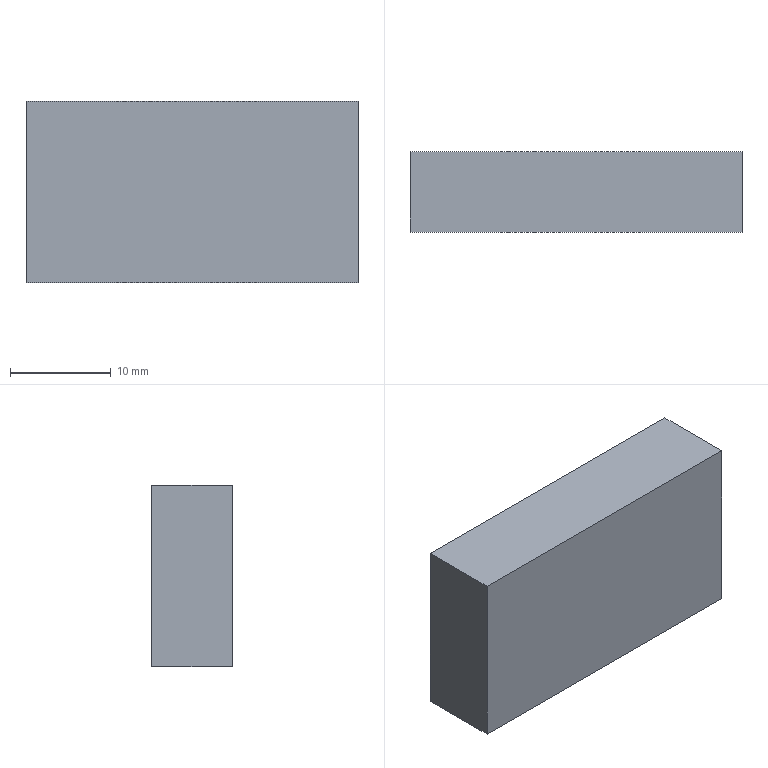Part | SolidWorks | features BaseBody 1 | 1 solid | 6 faces | box 33 x 8 x 18 mm | volume 4752 mm3 | plane 6
STEP:
#1=CARTESIAN_POINT('',(16.5,8.,9.));
#2=VERTEX_POINT('',#1);
#3=CARTESIAN_POINT('',(16.5,8.,-9.));
#4=VERTEX_POINT('',#3);
#5=CARTESIAN_POINT('',(16.5,8.,0.));
#6=DIRECTION('',(0.,0.,-1.));
#7=VECTOR('',#6,1000.);
#8=LINE('',#5,#7);
#9=EDGE_CURVE('',#2,#4,#8,.T.);
#10=ORIENTED_EDGE('',*,*,#9,.T.);
#11=CARTESIAN_POINT('',(-16.5,8.,-9.));
#12=VERTEX_POINT('',#11);
#13=CARTESIAN_POINT('',(0.,8.,-9.));
#14=DIRECTION('',(-1.,0.,0.));
#15=VECTOR('',#14,1000.);
#16=LINE('',#13,#15);
#17=EDGE_CURVE('',#4,#12,#16,.T.);
#18=ORIENTED_EDGE('',*,*,#17,.T.);
#19=CARTESIAN_POINT('',(-16.5,8.,9.));
#20=VERTEX_POINT('',#19);
#21=CARTESIAN_POINT('',(-16.5,8.,0.));
#22=DIRECTION('',(0.,0.,1.));
#23=VECTOR('',#22,1000.);
#24=LINE('',#21,#23);
#25=EDGE_CURVE('',#12,#20,#24,.T.);
#26=ORIENTED_EDGE('',*,*,#25,.T.);
#27=CARTESIAN_POINT('',(0.,8.,9.));
#28=DIRECTION('',(1.,0.,0.));
#29=VECTOR('',#28,1000.);
#30=LINE('',#27,#29);
#31=EDGE_CURVE('',#20,#2,#30,.T.);
#32=ORIENTED_EDGE('',*,*,#31,.T.);
#33=EDGE_LOOP('',(#10,#18,#26,#32));
#34=FACE_OUTER_BOUND('',#33,.T.);
#35=CARTESIAN_POINT('',(0.,8.,0.));
#36=DIRECTION('',(0.,1.,0.));
#37=DIRECTION('',(0.,0.,1.));
#38=AXIS2_PLACEMENT_3D('',#35,#36,#37);
#39=PLANE('',#38);
#40=ADVANCED_FACE('',(#34),#39,.T.);
#41=CARTESIAN_POINT('',(-16.5,0.,-9.));
#42=VERTEX_POINT('',#41);
#43=CARTESIAN_POINT('',(-16.5,8.,-9.));
#44=DIRECTION('',(0.,-1.,0.));
#45=VECTOR('',#44,1000.);
#46=LINE('',#43,#45);
#47=EDGE_CURVE('',#12,#42,#46,.T.);
#48=ORIENTED_EDGE('',*,*,#47,.F.);
#49=ORIENTED_EDGE('',*,*,#17,.F.);
#50=CARTESIAN_POINT('',(16.5,0.,-9.));
#51=VERTEX_POINT('',#50);
#52=CARTESIAN_POINT('',(16.5,8.,-9.));
#53=DIRECTION('',(0.,1.,0.));
#54=VECTOR('',#53,1000.);
#55=LINE('',#52,#54);
#56=EDGE_CURVE('',#51,#4,#55,.T.);
#57=ORIENTED_EDGE('',*,*,#56,.F.);
#58=CARTESIAN_POINT('',(16.5,0.,-9.));
#59=DIRECTION('',(1.,0.,0.));
#60=VECTOR('',#59,1000.);
#61=LINE('',#58,#60);
#62=EDGE_CURVE('',#42,#51,#61,.T.);
#63=ORIENTED_EDGE('',*,*,#62,.F.);
#64=EDGE_LOOP('',(#48,#49,#57,#63));
#65=FACE_OUTER_BOUND('',#64,.T.);
#66=CARTESIAN_POINT('',(16.5,8.,-9.));
#67=DIRECTION('',(0.,0.,1.));
#68=DIRECTION('',(1.,0.,0.));
#69=AXIS2_PLACEMENT_3D('',#66,#67,#68);
#70=PLANE('',#69);
#71=ADVANCED_FACE('',(#65),#70,.F.);
#72=ORIENTED_EDGE('',*,*,#56,.T.);
#73=ORIENTED_EDGE('',*,*,#9,.F.);
#74=CARTESIAN_POINT('',(16.5,0.,9.));
#75=VERTEX_POINT('',#74);
#76=CARTESIAN_POINT('',(16.5,8.,9.));
#77=DIRECTION('',(0.,1.,0.));
#78=VECTOR('',#77,1000.);
#79=LINE('',#76,#78);
#80=EDGE_CURVE('',#75,#2,#79,.T.);
#81=ORIENTED_EDGE('',*,*,#80,.F.);
#82=CARTESIAN_POINT('',(16.5,0.,9.));
#83=DIRECTION('',(0.,0.,1.));
#84=VECTOR('',#83,1000.);
#85=LINE('',#82,#84);
#86=EDGE_CURVE('',#51,#75,#85,.T.);
#87=ORIENTED_EDGE('',*,*,#86,.F.);
#88=EDGE_LOOP('',(#72,#73,#81,#87));
#89=FACE_OUTER_BOUND('',#88,.T.);
#90=CARTESIAN_POINT('',(16.5,8.,9.));
#91=DIRECTION('',(-1.,0.,0.));
#92=DIRECTION('',(0.,0.,1.));
#93=AXIS2_PLACEMENT_3D('',#90,#91,#92);
#94=PLANE('',#93);
#95=ADVANCED_FACE('',(#89),#94,.F.);
#96=ORIENTED_EDGE('',*,*,#80,.T.);
#97=ORIENTED_EDGE('',*,*,#31,.F.);
#98=CARTESIAN_POINT('',(-16.5,0.,9.));
#99=VERTEX_POINT('',#98);
#100=CARTESIAN_POINT('',(-16.5,8.,9.));
#101=DIRECTION('',(0.,1.,0.));
#102=VECTOR('',#101,1000.);
#103=LINE('',#100,#102);
#104=EDGE_CURVE('',#99,#20,#103,.T.);
#105=ORIENTED_EDGE('',*,*,#104,.F.);
#106=CARTESIAN_POINT('',(16.5,0.,9.));
#107=DIRECTION('',(-1.,0.,0.));
#108=VECTOR('',#107,1000.);
#109=LINE('',#106,#108);
#110=EDGE_CURVE('',#75,#99,#109,.T.);
#111=ORIENTED_EDGE('',*,*,#110,.F.);
#112=EDGE_LOOP('',(#96,#97,#105,#111));
#113=FACE_OUTER_BOUND('',#112,.T.);
#114=CARTESIAN_POINT('',(16.5,8.,9.));
#115=DIRECTION('',(0.,0.,-1.));
#116=DIRECTION('',(-1.,0.,0.));
#117=AXIS2_PLACEMENT_3D('',#114,#115,#116);
#118=PLANE('',#117);
#119=ADVANCED_FACE('',(#113),#118,.F.);
#120=ORIENTED_EDGE('',*,*,#104,.T.);
#121=ORIENTED_EDGE('',*,*,#25,.F.);
#122=ORIENTED_EDGE('',*,*,#47,.T.);
#123=CARTESIAN_POINT('',(-16.5,0.,9.));
#124=DIRECTION('',(0.,0.,-1.));
#125=VECTOR('',#124,1000.);
#126=LINE('',#123,#125);
#127=EDGE_CURVE('',#99,#42,#126,.T.);
#128=ORIENTED_EDGE('',*,*,#127,.F.);
#129=EDGE_LOOP('',(#120,#121,#122,#128));
#130=FACE_OUTER_BOUND('',#129,.T.);
#131=CARTESIAN_POINT('',(-16.5,8.,9.));
#132=DIRECTION('',(1.,0.,0.));
#133=DIRECTION('',(0.,0.,-1.));
#134=AXIS2_PLACEMENT_3D('',#131,#132,#133);
#135=PLANE('',#134);
#136=ADVANCED_FACE('',(#130),#135,.F.);
#137=ORIENTED_EDGE('',*,*,#62,.T.);
#138=ORIENTED_EDGE('',*,*,#86,.T.);
#139=ORIENTED_EDGE('',*,*,#110,.T.);
#140=ORIENTED_EDGE('',*,*,#127,.T.);
#141=EDGE_LOOP('',(#137,#138,#139,#140));
#142=FACE_OUTER_BOUND('',#141,.T.);
#143=CARTESIAN_POINT('',(0.,0.,0.));
#144=DIRECTION('',(0.,1.,0.));
#145=DIRECTION('',(0.,0.,1.));
#146=AXIS2_PLACEMENT_3D('',#143,#144,#145);
#147=PLANE('',#146);
#148=ADVANCED_FACE('',(#142),#147,.F.);
#149=CLOSED_SHELL('',(#40,#71,#95,#119,#136,#148));
#150=MANIFOLD_SOLID_BREP('',#149);
#151=CARTESIAN_POINT('',(0.,0.,0.));
#152=DIRECTION('',(0.,0.,1.));
#153=DIRECTION('',(1.,0.,0.));
#154=AXIS2_PLACEMENT_3D('',#151,#152,#153);
#155=(LENGTH_UNIT()NAMED_UNIT(*)SI_UNIT(.MILLI.,.METRE.));
#156=UNCERTAINTY_MEASURE_WITH_UNIT(LENGTH_MEASURE(0.00001),#155,'','');
#157=(NAMED_UNIT(*)PLANE_ANGLE_UNIT()SI_UNIT($,.RADIAN.));
#158=(NAMED_UNIT(*)SI_UNIT($,.STERADIAN.)SOLID_ANGLE_UNIT());
#159=(GEOMETRIC_REPRESENTATION_CONTEXT(3)GLOBAL_UNCERTAINTY_ASSIGNED_CONTEXT((#156))GLOBAL_UNIT_ASSIGNED_CONTEXT((#155,#157,#158))REPRESENTATION_CONTEXT('',''));
#160=ADVANCED_BREP_SHAPE_REPRESENTATION('',(#150,#154),#159);